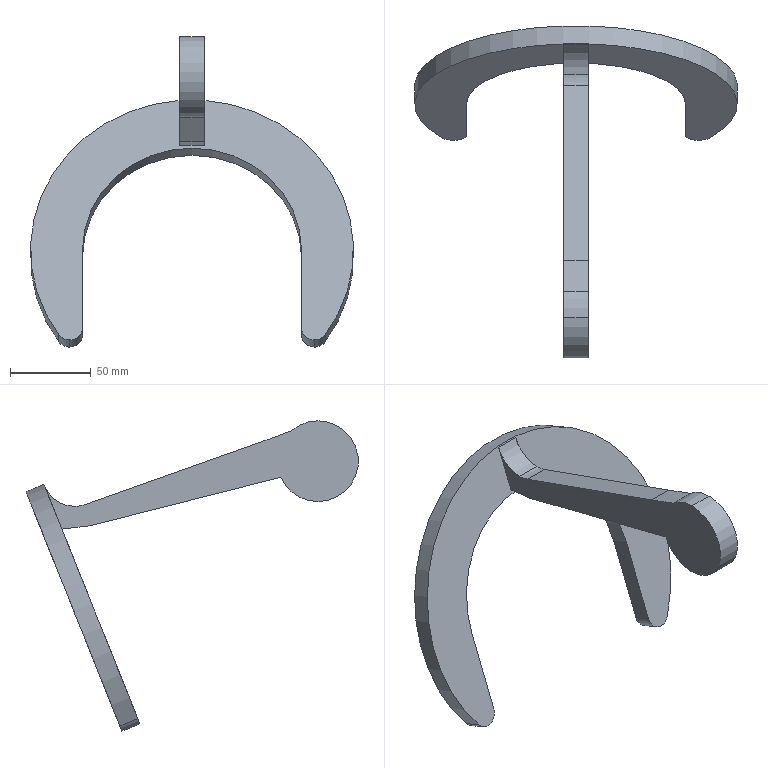Part | SolidWorks | features ICE 2, Extrusion 1, Fillet 1 | 1 solid | 21 faces | box 200 x 205.934 x 192.17 mm | volume 208238 mm3 | cylinder 11 | plane 10 | commonest cylinder face diameters 16 x4 50 x3 40 x2 135.704 x1 200 x1
STEP:
#1=CARTESIAN_POINT('',(-7.5,150.736,-27.917));
#2=VERTEX_POINT('',#1);
#3=CARTESIAN_POINT('',(-7.5,169.302,-15.355));
#4=VERTEX_POINT('',#3);
#5=CARTESIAN_POINT('',(-7.5,150.736,-7.917));
#6=DIRECTION('',(1.,0.,0.));
#7=DIRECTION('',(0.,0.,-1.));
#8=AXIS2_PLACEMENT_3D('',#5,#6,#7);
#9=CIRCLE('',#8,20.);
#10=EDGE_CURVE('',#2,#4,#9,.T.);
#11=ORIENTED_EDGE('',*,*,#10,.F.);
#12=CARTESIAN_POINT('',(7.5,150.736,-27.917));
#13=VERTEX_POINT('',#12);
#14=CARTESIAN_POINT('',(7.5,150.736,-27.917));
#15=DIRECTION('',(1.,0.,0.));
#16=VECTOR('',#15,1000.);
#17=LINE('',#14,#16);
#18=EDGE_CURVE('',#2,#13,#17,.T.);
#19=ORIENTED_EDGE('',*,*,#18,.T.);
#20=CARTESIAN_POINT('',(7.5,169.302,-15.355));
#21=VERTEX_POINT('',#20);
#22=CARTESIAN_POINT('',(7.5,150.736,-7.917));
#23=DIRECTION('',(-1.,0.,0.));
#24=DIRECTION('',(0.,0.,-1.));
#25=AXIS2_PLACEMENT_3D('',#22,#23,#24);
#26=CIRCLE('',#25,20.);
#27=EDGE_CURVE('',#21,#13,#26,.T.);
#28=ORIENTED_EDGE('',*,*,#27,.F.);
#29=CARTESIAN_POINT('',(7.5,169.302,-15.355));
#30=DIRECTION('',(1.,0.,0.));
#31=VECTOR('',#30,1000.);
#32=LINE('',#29,#31);
#33=EDGE_CURVE('',#4,#21,#32,.T.);
#34=ORIENTED_EDGE('',*,*,#33,.F.);
#35=EDGE_LOOP('',(#11,#19,#28,#34));
#36=FACE_OUTER_BOUND('',#35,.T.);
#37=CARTESIAN_POINT('',(7.5,150.736,-7.917));
#38=DIRECTION('',(1.,0.,0.));
#39=DIRECTION('',(0.,0.,-1.));
#40=AXIS2_PLACEMENT_3D('',#37,#38,#39);
#41=CYLINDRICAL_SURFACE('',#40,20.);
#42=ADVANCED_FACE('',(#36),#41,.F.);
#43=CARTESIAN_POINT('',(75.852,121.408,-167.17));
#44=VERTEX_POINT('',#43);
#45=CARTESIAN_POINT('',(67.852,124.383,-159.743));
#46=VERTEX_POINT('',#45);
#47=CARTESIAN_POINT('',(75.852,124.383,-159.743));
#48=DIRECTION('',(0.,0.9283,-0.3719));
#49=DIRECTION('',(0.,-0.3719,-0.9283));
#50=AXIS2_PLACEMENT_3D('',#47,#48,#49);
#51=CIRCLE('',#50,8.);
#52=EDGE_CURVE('',#44,#46,#51,.T.);
#53=ORIENTED_EDGE('',*,*,#52,.F.);
#54=CARTESIAN_POINT('',(75.852,110.269,-162.707));
#55=VERTEX_POINT('',#54);
#56=CARTESIAN_POINT('',(75.852,121.408,-167.17));
#57=DIRECTION('',(0.,-0.9283,0.3719));
#58=VECTOR('',#57,1000.);
#59=LINE('',#56,#58);
#60=EDGE_CURVE('',#44,#55,#59,.T.);
#61=ORIENTED_EDGE('',*,*,#60,.T.);
#62=CARTESIAN_POINT('',(67.852,113.244,-155.281));
#63=VERTEX_POINT('',#62);
#64=CARTESIAN_POINT('',(75.852,113.244,-155.281));
#65=DIRECTION('',(0.,0.9283,-0.3719));
#66=DIRECTION('',(0.,-0.3719,-0.9283));
#67=AXIS2_PLACEMENT_3D('',#64,#65,#66);
#68=CIRCLE('',#67,8.);
#69=EDGE_CURVE('',#55,#63,#68,.T.);
#70=ORIENTED_EDGE('',*,*,#69,.T.);
#71=CARTESIAN_POINT('',(67.852,124.383,-159.743));
#72=DIRECTION('',(0.,-0.9283,0.3719));
#73=VECTOR('',#72,1000.);
#74=LINE('',#71,#73);
#75=EDGE_CURVE('',#46,#63,#74,.T.);
#76=ORIENTED_EDGE('',*,*,#75,.F.);
#77=EDGE_LOOP('',(#53,#61,#70,#76));
#78=FACE_OUTER_BOUND('',#77,.T.);
#79=CARTESIAN_POINT('',(75.852,124.383,-159.743));
#80=DIRECTION('',(0.,-0.9283,0.3719));
#81=DIRECTION('',(0.,-0.3719,-0.9283));
#82=AXIS2_PLACEMENT_3D('',#79,#80,#81);
#83=CYLINDRICAL_SURFACE('',#82,8.);
#84=ADVANCED_FACE('',(#78),#83,.T.);
#85=CARTESIAN_POINT('',(-75.852,121.408,-167.17));
#86=VERTEX_POINT('',#85);
#87=CARTESIAN_POINT('',(-82.448,122.7,-163.946));
#88=VERTEX_POINT('',#87);
#89=CARTESIAN_POINT('',(-75.852,124.383,-159.743));
#90=DIRECTION('',(0.,0.9283,-0.3719));
#91=DIRECTION('',(0.,0.3719,0.9283));
#92=AXIS2_PLACEMENT_3D('',#89,#90,#91);
#93=CIRCLE('',#92,8.);
#94=EDGE_CURVE('',#86,#88,#93,.T.);
#95=ORIENTED_EDGE('',*,*,#94,.F.);
#96=CARTESIAN_POINT('',(-75.852,110.269,-162.707));
#97=VERTEX_POINT('',#96);
#98=CARTESIAN_POINT('',(-75.852,121.408,-167.17));
#99=DIRECTION('',(0.,-0.9283,0.3719));
#100=VECTOR('',#99,1000.);
#101=LINE('',#98,#100);
#102=EDGE_CURVE('',#86,#97,#101,.T.);
#103=ORIENTED_EDGE('',*,*,#102,.T.);
#104=CARTESIAN_POINT('',(-82.448,111.56,-159.483));
#105=VERTEX_POINT('',#104);
#106=CARTESIAN_POINT('',(-75.852,113.244,-155.281));
#107=DIRECTION('',(0.,0.9283,-0.3719));
#108=DIRECTION('',(0.,0.3719,0.9283));
#109=AXIS2_PLACEMENT_3D('',#106,#107,#108);
#110=CIRCLE('',#109,8.);
#111=EDGE_CURVE('',#97,#105,#110,.T.);
#112=ORIENTED_EDGE('',*,*,#111,.T.);
#113=CARTESIAN_POINT('',(-82.448,122.7,-163.946));
#114=DIRECTION('',(0.,-0.9283,0.3719));
#115=VECTOR('',#114,1000.);
#116=LINE('',#113,#115);
#117=EDGE_CURVE('',#88,#105,#116,.T.);
#118=ORIENTED_EDGE('',*,*,#117,.F.);
#119=EDGE_LOOP('',(#95,#103,#112,#118));
#120=FACE_OUTER_BOUND('',#119,.T.);
#121=CARTESIAN_POINT('',(-75.852,124.383,-159.743));
#122=DIRECTION('',(0.,-0.9283,0.3719));
#123=DIRECTION('',(0.,-0.3719,-0.9283));
#124=AXIS2_PLACEMENT_3D('',#121,#122,#123);
#125=CYLINDRICAL_SURFACE('',#124,8.);
#126=ADVANCED_FACE('',(#120),#125,.T.);
#127=CARTESIAN_POINT('',(7.5,0.,-25.));
#128=VERTEX_POINT('',#127);
#129=CARTESIAN_POINT('',(7.5,22.922,-9.978));
#130=VERTEX_POINT('',#129);
#131=CARTESIAN_POINT('',(7.5,0.,0.));
#132=DIRECTION('',(1.,0.,0.));
#133=DIRECTION('',(0.,0.,-1.));
#134=AXIS2_PLACEMENT_3D('',#131,#132,#133);
#135=CIRCLE('',#134,25.);
#136=EDGE_CURVE('',#128,#130,#135,.T.);
#137=ORIENTED_EDGE('',*,*,#136,.F.);
#138=CARTESIAN_POINT('',(-7.5,0.,-25.));
#139=VERTEX_POINT('',#138);
#140=CARTESIAN_POINT('',(7.5,0.,-25.));
#141=DIRECTION('',(-1.,0.,0.));
#142=VECTOR('',#141,1000.);
#143=LINE('',#140,#142);
#144=EDGE_CURVE('',#128,#139,#143,.T.);
#145=ORIENTED_EDGE('',*,*,#144,.T.);
#146=CARTESIAN_POINT('',(-7.5,22.922,-9.978));
#147=VERTEX_POINT('',#146);
#148=CARTESIAN_POINT('',(-7.5,0.,0.));
#149=DIRECTION('',(1.,0.,0.));
#150=DIRECTION('',(0.,0.,-1.));
#151=AXIS2_PLACEMENT_3D('',#148,#149,#150);
#152=CIRCLE('',#151,25.);
#153=EDGE_CURVE('',#139,#147,#152,.T.);
#154=ORIENTED_EDGE('',*,*,#153,.T.);
#155=CARTESIAN_POINT('',(7.5,22.922,-9.978));
#156=DIRECTION('',(-1.,0.,0.));
#157=VECTOR('',#156,1000.);
#158=LINE('',#155,#157);
#159=EDGE_CURVE('',#130,#147,#158,.T.);
#160=ORIENTED_EDGE('',*,*,#159,.F.);
#161=EDGE_LOOP('',(#137,#145,#154,#160));
#162=FACE_OUTER_BOUND('',#161,.T.);
#163=CARTESIAN_POINT('',(7.5,0.,0.));
#164=DIRECTION('',(-1.,0.,0.));
#165=DIRECTION('',(0.,0.,1.));
#166=AXIS2_PLACEMENT_3D('',#163,#164,#165);
#167=CYLINDRICAL_SURFACE('',#166,25.);
#168=ADVANCED_FACE('',(#162),#167,.T.);
#169=ORIENTED_EDGE('',*,*,#144,.F.);
#170=CARTESIAN_POINT('',(7.5,0.,25.));
#171=VERTEX_POINT('',#170);
#172=CARTESIAN_POINT('',(7.5,0.,0.));
#173=DIRECTION('',(1.,0.,0.));
#174=DIRECTION('',(0.,0.,-1.));
#175=AXIS2_PLACEMENT_3D('',#172,#173,#174);
#176=CIRCLE('',#175,25.);
#177=EDGE_CURVE('',#171,#128,#176,.T.);
#178=ORIENTED_EDGE('',*,*,#177,.F.);
#179=CARTESIAN_POINT('',(-7.5,0.,25.));
#180=VERTEX_POINT('',#179);
#181=CARTESIAN_POINT('',(7.5,0.,25.));
#182=DIRECTION('',(-1.,0.,0.));
#183=VECTOR('',#182,1000.);
#184=LINE('',#181,#183);
#185=EDGE_CURVE('',#171,#180,#184,.T.);
#186=ORIENTED_EDGE('',*,*,#185,.T.);
#187=CARTESIAN_POINT('',(-7.5,0.,0.));
#188=DIRECTION('',(1.,0.,0.));
#189=DIRECTION('',(0.,0.,-1.));
#190=AXIS2_PLACEMENT_3D('',#187,#188,#189);
#191=CIRCLE('',#190,25.);
#192=EDGE_CURVE('',#180,#139,#191,.T.);
#193=ORIENTED_EDGE('',*,*,#192,.T.);
#194=EDGE_LOOP('',(#169,#178,#186,#193));
#195=FACE_OUTER_BOUND('',#194,.T.);
#196=CARTESIAN_POINT('',(7.5,0.,0.));
#197=DIRECTION('',(-1.,0.,0.));
#198=DIRECTION('',(0.,0.,1.));
#199=AXIS2_PLACEMENT_3D('',#196,#197,#198);
#200=CYLINDRICAL_SURFACE('',#199,25.);
#201=ADVANCED_FACE('',(#195),#200,.T.);
#202=ORIENTED_EDGE('',*,*,#185,.F.);
#203=CARTESIAN_POINT('',(7.5,16.342,18.92));
#204=VERTEX_POINT('',#203);
#205=CARTESIAN_POINT('',(7.5,0.,0.));
#206=DIRECTION('',(1.,0.,0.));
#207=DIRECTION('',(0.,0.,-1.));
#208=AXIS2_PLACEMENT_3D('',#205,#206,#207);
#209=CIRCLE('',#208,25.);
#210=EDGE_CURVE('',#204,#171,#209,.T.);
#211=ORIENTED_EDGE('',*,*,#210,.F.);
#212=CARTESIAN_POINT('',(-7.5,16.342,18.92));
#213=VERTEX_POINT('',#212);
#214=CARTESIAN_POINT('',(7.5,16.342,18.92));
#215=DIRECTION('',(1.,0.,0.));
#216=VECTOR('',#215,1000.);
#217=LINE('',#214,#216);
#218=EDGE_CURVE('',#213,#204,#217,.T.);
#219=ORIENTED_EDGE('',*,*,#218,.F.);
#220=CARTESIAN_POINT('',(-7.5,0.,0.));
#221=DIRECTION('',(1.,0.,0.));
#222=DIRECTION('',(0.,0.,-1.));
#223=AXIS2_PLACEMENT_3D('',#220,#221,#222);
#224=CIRCLE('',#223,25.);
#225=EDGE_CURVE('',#213,#180,#224,.T.);
#226=ORIENTED_EDGE('',*,*,#225,.T.);
#227=EDGE_LOOP('',(#202,#211,#219,#226));
#228=FACE_OUTER_BOUND('',#227,.T.);
#229=CARTESIAN_POINT('',(7.5,0.,0.));
#230=DIRECTION('',(-1.,0.,0.));
#231=DIRECTION('',(0.,0.,1.));
#232=AXIS2_PLACEMENT_3D('',#229,#230,#231);
#233=CYLINDRICAL_SURFACE('',#232,25.);
#234=ADVANCED_FACE('',(#228),#233,.T.);
#235=ORIENTED_EDGE('',*,*,#210,.T.);
#236=ORIENTED_EDGE('',*,*,#177,.T.);
#237=ORIENTED_EDGE('',*,*,#136,.T.);
#238=CARTESIAN_POINT('',(7.5,141.125,-39.917));
#239=VERTEX_POINT('',#238);
#240=CARTESIAN_POINT('',(7.5,-2.,-3.666));
#241=DIRECTION('',(0.,0.9694,-0.2455));
#242=VECTOR('',#241,1000.);
#243=LINE('',#240,#242);
#244=EDGE_CURVE('',#130,#239,#243,.T.);
#245=ORIENTED_EDGE('',*,*,#244,.T.);
#246=CARTESIAN_POINT('',(7.5,158.581,-42.115));
#247=VERTEX_POINT('',#246);
#248=CARTESIAN_POINT('',(7.5,141.125,-39.917));
#249=DIRECTION('',(0.,0.9922,-0.1249));
#250=VECTOR('',#249,1000.);
#251=LINE('',#248,#250);
#252=EDGE_CURVE('',#239,#247,#251,.T.);
#253=ORIENTED_EDGE('',*,*,#252,.T.);
#254=CARTESIAN_POINT('',(7.5,158.581,-42.115));
#255=DIRECTION('',(0.,0.3719,0.9283));
#256=VECTOR('',#255,1000.);
#257=LINE('',#254,#256);
#258=EDGE_CURVE('',#247,#21,#257,.T.);
#259=ORIENTED_EDGE('',*,*,#258,.T.);
#260=ORIENTED_EDGE('',*,*,#27,.T.);
#261=CARTESIAN_POINT('',(7.5,144.041,-26.763));
#262=VERTEX_POINT('',#261);
#263=CARTESIAN_POINT('',(7.5,150.736,-7.917));
#264=DIRECTION('',(-1.,0.,0.));
#265=DIRECTION('',(0.,0.,-1.));
#266=AXIS2_PLACEMENT_3D('',#263,#264,#265);
#267=CIRCLE('',#266,20.);
#268=EDGE_CURVE('',#13,#262,#267,.T.);
#269=ORIENTED_EDGE('',*,*,#268,.T.);
#270=CARTESIAN_POINT('',(7.5,35.334,11.853));
#271=VERTEX_POINT('',#270);
#272=CARTESIAN_POINT('',(7.5,35.334,11.853));
#273=DIRECTION('',(0.,-0.9423,0.3347));
#274=VECTOR('',#273,1000.);
#275=LINE('',#272,#274);
#276=EDGE_CURVE('',#262,#271,#275,.T.);
#277=ORIENTED_EDGE('',*,*,#276,.T.);
#278=CARTESIAN_POINT('',(7.5,0.,25.));
#279=DIRECTION('',(0.,-0.9372,0.3487));
#280=VECTOR('',#279,1000.);
#281=LINE('',#278,#280);
#282=EDGE_CURVE('',#271,#204,#281,.T.);
#283=ORIENTED_EDGE('',*,*,#282,.T.);
#284=EDGE_LOOP('',(#235,#236,#237,#245,#253,#259,#260,#269,#277,#283));
#285=FACE_OUTER_BOUND('',#284,.T.);
#286=CARTESIAN_POINT('',(7.5,0.,0.));
#287=DIRECTION('',(1.,0.,0.));
#288=DIRECTION('',(0.,0.,-1.));
#289=AXIS2_PLACEMENT_3D('',#286,#287,#288);
#290=PLANE('',#289);
#291=ADVANCED_FACE('',(#285),#290,.T.);
#292=CARTESIAN_POINT('',(-7.5,141.125,-39.917));
#293=VERTEX_POINT('',#292);
#294=CARTESIAN_POINT('',(-7.5,-2.,-3.666));
#295=DIRECTION('',(0.,0.9694,-0.2455));
#296=VECTOR('',#295,1000.);
#297=LINE('',#294,#296);
#298=EDGE_CURVE('',#147,#293,#297,.T.);
#299=ORIENTED_EDGE('',*,*,#298,.F.);
#300=ORIENTED_EDGE('',*,*,#153,.F.);
#301=ORIENTED_EDGE('',*,*,#192,.F.);
#302=ORIENTED_EDGE('',*,*,#225,.F.);
#303=CARTESIAN_POINT('',(-7.5,35.334,11.853));
#304=VERTEX_POINT('',#303);
#305=CARTESIAN_POINT('',(-7.5,0.,25.));
#306=DIRECTION('',(0.,-0.9372,0.3487));
#307=VECTOR('',#306,1000.);
#308=LINE('',#305,#307);
#309=EDGE_CURVE('',#304,#213,#308,.T.);
#310=ORIENTED_EDGE('',*,*,#309,.F.);
#311=CARTESIAN_POINT('',(-7.5,144.041,-26.763));
#312=VERTEX_POINT('',#311);
#313=CARTESIAN_POINT('',(-7.5,35.334,11.853));
#314=DIRECTION('',(0.,-0.9423,0.3347));
#315=VECTOR('',#314,1000.);
#316=LINE('',#313,#315);
#317=EDGE_CURVE('',#312,#304,#316,.T.);
#318=ORIENTED_EDGE('',*,*,#317,.F.);
#319=CARTESIAN_POINT('',(-7.5,150.736,-7.917));
#320=DIRECTION('',(1.,0.,0.));
#321=DIRECTION('',(0.,0.,-1.));
#322=AXIS2_PLACEMENT_3D('',#319,#320,#321);
#323=CIRCLE('',#322,20.);
#324=EDGE_CURVE('',#312,#2,#323,.T.);
#325=ORIENTED_EDGE('',*,*,#324,.T.);
#326=ORIENTED_EDGE('',*,*,#10,.T.);
#327=CARTESIAN_POINT('',(-7.5,158.581,-42.115));
#328=VERTEX_POINT('',#327);
#329=CARTESIAN_POINT('',(-7.5,158.581,-42.115));
#330=DIRECTION('',(0.,0.3719,0.9283));
#331=VECTOR('',#330,1000.);
#332=LINE('',#329,#331);
#333=EDGE_CURVE('',#328,#4,#332,.T.);
#334=ORIENTED_EDGE('',*,*,#333,.F.);
#335=CARTESIAN_POINT('',(-7.5,141.125,-39.917));
#336=DIRECTION('',(0.,0.9922,-0.1249));
#337=VECTOR('',#336,1000.);
#338=LINE('',#335,#337);
#339=EDGE_CURVE('',#293,#328,#338,.T.);
#340=ORIENTED_EDGE('',*,*,#339,.F.);
#341=EDGE_LOOP('',(#299,#300,#301,#302,#310,#318,#325,#326,#334,#340));
#342=FACE_OUTER_BOUND('',#341,.T.);
#343=CARTESIAN_POINT('',(-7.5,0.,0.));
#344=DIRECTION('',(1.,0.,0.));
#345=DIRECTION('',(0.,0.,-1.));
#346=AXIS2_PLACEMENT_3D('',#343,#344,#345);
#347=PLANE('',#346);
#348=ADVANCED_FACE('',(#342),#347,.F.);
#349=ORIENTED_EDGE('',*,*,#244,.F.);
#350=ORIENTED_EDGE('',*,*,#159,.T.);
#351=ORIENTED_EDGE('',*,*,#298,.T.);
#352=CARTESIAN_POINT('',(7.5,141.125,-39.917));
#353=DIRECTION('',(-1.,0.,0.));
#354=VECTOR('',#353,1000.);
#355=LINE('',#352,#354);
#356=EDGE_CURVE('',#239,#293,#355,.T.);
#357=ORIENTED_EDGE('',*,*,#356,.F.);
#358=EDGE_LOOP('',(#349,#350,#351,#357));
#359=FACE_OUTER_BOUND('',#358,.T.);
#360=CARTESIAN_POINT('',(7.5,-2.,-3.666));
#361=DIRECTION('',(0.,0.2455,0.9694));
#362=DIRECTION('',(0.,-0.9694,0.2455));
#363=AXIS2_PLACEMENT_3D('',#360,#361,#362);
#364=PLANE('',#363);
#365=ADVANCED_FACE('',(#359),#364,.F.);
#366=ORIENTED_EDGE('',*,*,#309,.T.);
#367=ORIENTED_EDGE('',*,*,#218,.T.);
#368=ORIENTED_EDGE('',*,*,#282,.F.);
#369=CARTESIAN_POINT('',(7.5,35.334,11.853));
#370=DIRECTION('',(-1.,0.,0.));
#371=VECTOR('',#370,1000.);
#372=LINE('',#369,#371);
#373=EDGE_CURVE('',#271,#304,#372,.T.);
#374=ORIENTED_EDGE('',*,*,#373,.T.);
#375=EDGE_LOOP('',(#366,#367,#368,#374));
#376=FACE_OUTER_BOUND('',#375,.T.);
#377=CARTESIAN_POINT('',(7.5,0.,25.));
#378=DIRECTION('',(0.,-0.3487,-0.9372));
#379=DIRECTION('',(0.,0.9372,-0.3487));
#380=AXIS2_PLACEMENT_3D('',#377,#378,#379);
#381=PLANE('',#380);
#382=ADVANCED_FACE('',(#376),#381,.F.);
#383=ORIENTED_EDGE('',*,*,#339,.T.);
#384=CARTESIAN_POINT('',(7.5,158.581,-42.115));
#385=DIRECTION('',(-1.,0.,0.));
#386=VECTOR('',#385,1000.);
#387=LINE('',#384,#386);
#388=EDGE_CURVE('',#247,#328,#387,.T.);
#389=ORIENTED_EDGE('',*,*,#388,.F.);
#390=ORIENTED_EDGE('',*,*,#252,.F.);
#391=ORIENTED_EDGE('',*,*,#356,.T.);
#392=EDGE_LOOP('',(#383,#389,#390,#391));
#393=FACE_OUTER_BOUND('',#392,.T.);
#394=CARTESIAN_POINT('',(7.5,141.125,-39.917));
#395=DIRECTION('',(0.,0.1249,0.9922));
#396=DIRECTION('',(0.,-0.9922,0.1249));
#397=AXIS2_PLACEMENT_3D('',#394,#395,#396);
#398=PLANE('',#397);
#399=ADVANCED_FACE('',(#393),#398,.F.);
#400=ORIENTED_EDGE('',*,*,#276,.F.);
#401=CARTESIAN_POINT('',(-7.5,144.041,-26.763));
#402=DIRECTION('',(-1.,0.,0.));
#403=VECTOR('',#402,1000.);
#404=LINE('',#401,#403);
#405=EDGE_CURVE('',#262,#312,#404,.T.);
#406=ORIENTED_EDGE('',*,*,#405,.T.);
#407=ORIENTED_EDGE('',*,*,#317,.T.);
#408=ORIENTED_EDGE('',*,*,#373,.F.);
#409=EDGE_LOOP('',(#400,#406,#407,#408));
#410=FACE_OUTER_BOUND('',#409,.T.);
#411=CARTESIAN_POINT('',(7.5,35.334,11.853));
#412=DIRECTION('',(0.,-0.3347,-0.9423));
#413=DIRECTION('',(0.,0.9423,-0.3347));
#414=AXIS2_PLACEMENT_3D('',#411,#412,#413);
#415=PLANE('',#414);
#416=ADVANCED_FACE('',(#410),#415,.F.);
#417=CARTESIAN_POINT('',(-67.852,113.244,-155.281));
#418=VERTEX_POINT('',#417);
#419=CARTESIAN_POINT('',(-75.852,113.244,-155.281));
#420=DIRECTION('',(0.,0.9283,-0.3719));
#421=DIRECTION('',(0.,0.3719,0.9283));
#422=AXIS2_PLACEMENT_3D('',#419,#420,#421);
#423=CIRCLE('',#422,8.);
#424=EDGE_CURVE('',#418,#97,#423,.T.);
#425=ORIENTED_EDGE('',*,*,#424,.F.);
#426=CARTESIAN_POINT('',(-67.852,132.605,-106.953));
#427=VERTEX_POINT('',#426);
#428=CARTESIAN_POINT('',(-67.852,113.244,-155.281));
#429=DIRECTION('',(0.,-0.3719,-0.9283));
#430=VECTOR('',#429,1000.);
#431=LINE('',#428,#430);
#432=EDGE_CURVE('',#427,#418,#431,.T.);
#433=ORIENTED_EDGE('',*,*,#432,.F.);
#434=CARTESIAN_POINT('',(67.852,132.605,-106.953));
#435=VERTEX_POINT('',#434);
#436=CARTESIAN_POINT('',(0.,132.605,-106.953));
#437=DIRECTION('',(0.,-0.9283,0.3719));
#438=DIRECTION('',(0.,0.3719,0.9283));
#439=AXIS2_PLACEMENT_3D('',#436,#437,#438);
#440=CIRCLE('',#439,67.852);
#441=EDGE_CURVE('',#435,#427,#440,.T.);
#442=ORIENTED_EDGE('',*,*,#441,.F.);
#443=CARTESIAN_POINT('',(67.852,113.244,-155.281));
#444=DIRECTION('',(0.,0.3719,0.9283));
#445=VECTOR('',#444,1000.);
#446=LINE('',#443,#445);
#447=EDGE_CURVE('',#63,#435,#446,.T.);
#448=ORIENTED_EDGE('',*,*,#447,.F.);
#449=ORIENTED_EDGE('',*,*,#69,.F.);
#450=CARTESIAN_POINT('',(82.448,111.56,-159.483));
#451=VERTEX_POINT('',#450);
#452=CARTESIAN_POINT('',(75.852,113.244,-155.281));
#453=DIRECTION('',(0.,0.9283,-0.3719));
#454=DIRECTION('',(0.,-0.3719,-0.9283));
#455=AXIS2_PLACEMENT_3D('',#452,#453,#454);
#456=CIRCLE('',#455,8.);
#457=EDGE_CURVE('',#451,#55,#456,.T.);
#458=ORIENTED_EDGE('',*,*,#457,.F.);
#459=CARTESIAN_POINT('',(0.,132.605,-106.953));
#460=DIRECTION('',(0.,0.9283,-0.3719));
#461=DIRECTION('',(0.,0.3719,0.9283));
#462=AXIS2_PLACEMENT_3D('',#459,#460,#461);
#463=CIRCLE('',#462,100.);
#464=EDGE_CURVE('',#105,#451,#463,.T.);
#465=ORIENTED_EDGE('',*,*,#464,.F.);
#466=ORIENTED_EDGE('',*,*,#111,.F.);
#467=EDGE_LOOP('',(#425,#433,#442,#448,#449,#458,#465,#466));
#468=FACE_OUTER_BOUND('',#467,.T.);
#469=ORIENTED_EDGE('',*,*,#333,.T.);
#470=ORIENTED_EDGE('',*,*,#33,.T.);
#471=ORIENTED_EDGE('',*,*,#258,.F.);
#472=ORIENTED_EDGE('',*,*,#388,.T.);
#473=EDGE_LOOP('',(#469,#470,#471,#472));
#474=FACE_BOUND('',#473,.T.);
#475=CARTESIAN_POINT('',(-75.852,113.244,-155.281));
#476=DIRECTION('',(0.,0.9283,-0.3719));
#477=DIRECTION('',(0.,0.3719,0.9283));
#478=AXIS2_PLACEMENT_3D('',#475,#476,#477);
#479=PLANE('',#478);
#480=ADVANCED_FACE('',(#468,#474),#479,.F.);
#481=ORIENTED_EDGE('',*,*,#102,.F.);
#482=CARTESIAN_POINT('',(-67.852,124.383,-159.743));
#483=VERTEX_POINT('',#482);
#484=CARTESIAN_POINT('',(-75.852,124.383,-159.743));
#485=DIRECTION('',(0.,0.9283,-0.3719));
#486=DIRECTION('',(0.,0.3719,0.9283));
#487=AXIS2_PLACEMENT_3D('',#484,#485,#486);
#488=CIRCLE('',#487,8.);
#489=EDGE_CURVE('',#483,#86,#488,.T.);
#490=ORIENTED_EDGE('',*,*,#489,.F.);
#491=CARTESIAN_POINT('',(-67.852,124.383,-159.743));
#492=DIRECTION('',(0.,-0.9283,0.3719));
#493=VECTOR('',#492,1000.);
#494=LINE('',#491,#493);
#495=EDGE_CURVE('',#483,#418,#494,.T.);
#496=ORIENTED_EDGE('',*,*,#495,.T.);
#497=ORIENTED_EDGE('',*,*,#424,.T.);
#498=EDGE_LOOP('',(#481,#490,#496,#497));
#499=FACE_OUTER_BOUND('',#498,.T.);
#500=CARTESIAN_POINT('',(-75.852,124.383,-159.743));
#501=DIRECTION('',(0.,-0.9283,0.3719));
#502=DIRECTION('',(0.,-0.3719,-0.9283));
#503=AXIS2_PLACEMENT_3D('',#500,#501,#502);
#504=CYLINDRICAL_SURFACE('',#503,8.);
#505=ADVANCED_FACE('',(#499),#504,.T.);
#506=ORIENTED_EDGE('',*,*,#464,.T.);
#507=CARTESIAN_POINT('',(82.448,122.7,-163.946));
#508=VERTEX_POINT('',#507);
#509=CARTESIAN_POINT('',(82.448,122.7,-163.946));
#510=DIRECTION('',(0.,-0.9283,0.3719));
#511=VECTOR('',#510,1000.);
#512=LINE('',#509,#511);
#513=EDGE_CURVE('',#508,#451,#512,.T.);
#514=ORIENTED_EDGE('',*,*,#513,.F.);
#515=CARTESIAN_POINT('',(0.,143.745,-111.415));
#516=DIRECTION('',(0.,0.9283,-0.3719));
#517=DIRECTION('',(0.,0.3719,0.9283));
#518=AXIS2_PLACEMENT_3D('',#515,#516,#517);
#519=CIRCLE('',#518,100.);
#520=EDGE_CURVE('',#88,#508,#519,.T.);
#521=ORIENTED_EDGE('',*,*,#520,.F.);
#522=ORIENTED_EDGE('',*,*,#117,.T.);
#523=EDGE_LOOP('',(#506,#514,#521,#522));
#524=FACE_OUTER_BOUND('',#523,.T.);
#525=CARTESIAN_POINT('',(0.,143.745,-111.415));
#526=DIRECTION('',(0.,-0.9283,0.3719));
#527=DIRECTION('',(0.,-0.3719,-0.9283));
#528=AXIS2_PLACEMENT_3D('',#525,#526,#527);
#529=CYLINDRICAL_SURFACE('',#528,100.);
#530=ADVANCED_FACE('',(#524),#529,.T.);
#531=ORIENTED_EDGE('',*,*,#60,.F.);
#532=CARTESIAN_POINT('',(75.852,124.383,-159.743));
#533=DIRECTION('',(0.,0.9283,-0.3719));
#534=DIRECTION('',(0.,-0.3719,-0.9283));
#535=AXIS2_PLACEMENT_3D('',#532,#533,#534);
#536=CIRCLE('',#535,8.);
#537=EDGE_CURVE('',#508,#44,#536,.T.);
#538=ORIENTED_EDGE('',*,*,#537,.F.);
#539=ORIENTED_EDGE('',*,*,#513,.T.);
#540=ORIENTED_EDGE('',*,*,#457,.T.);
#541=EDGE_LOOP('',(#531,#538,#539,#540));
#542=FACE_OUTER_BOUND('',#541,.T.);
#543=CARTESIAN_POINT('',(75.852,124.383,-159.743));
#544=DIRECTION('',(0.,-0.9283,0.3719));
#545=DIRECTION('',(0.,-0.3719,-0.9283));
#546=AXIS2_PLACEMENT_3D('',#543,#544,#545);
#547=CYLINDRICAL_SURFACE('',#546,8.);
#548=ADVANCED_FACE('',(#542),#547,.T.);
#549=ORIENTED_EDGE('',*,*,#447,.T.);
#550=CARTESIAN_POINT('',(67.852,143.745,-111.415));
#551=VERTEX_POINT('',#550);
#552=CARTESIAN_POINT('',(67.852,143.745,-111.415));
#553=DIRECTION('',(0.,-0.9283,0.3719));
#554=VECTOR('',#553,1000.);
#555=LINE('',#552,#554);
#556=EDGE_CURVE('',#551,#435,#555,.T.);
#557=ORIENTED_EDGE('',*,*,#556,.F.);
#558=CARTESIAN_POINT('',(67.852,124.383,-159.743));
#559=DIRECTION('',(0.,0.3719,0.9283));
#560=VECTOR('',#559,1000.);
#561=LINE('',#558,#560);
#562=EDGE_CURVE('',#46,#551,#561,.T.);
#563=ORIENTED_EDGE('',*,*,#562,.F.);
#564=ORIENTED_EDGE('',*,*,#75,.T.);
#565=EDGE_LOOP('',(#549,#557,#563,#564));
#566=FACE_OUTER_BOUND('',#565,.T.);
#567=CARTESIAN_POINT('',(67.852,124.383,-159.743));
#568=DIRECTION('',(1.,0.,0.));
#569=DIRECTION('',(0.,0.,-1.));
#570=AXIS2_PLACEMENT_3D('',#567,#568,#569);
#571=PLANE('',#570);
#572=ADVANCED_FACE('',(#566),#571,.F.);
#573=ORIENTED_EDGE('',*,*,#441,.T.);
#574=CARTESIAN_POINT('',(-67.852,143.745,-111.415));
#575=VERTEX_POINT('',#574);
#576=CARTESIAN_POINT('',(-67.852,143.745,-111.415));
#577=DIRECTION('',(0.,-0.9283,0.3719));
#578=VECTOR('',#577,1000.);
#579=LINE('',#576,#578);
#580=EDGE_CURVE('',#575,#427,#579,.T.);
#581=ORIENTED_EDGE('',*,*,#580,.F.);
#582=CARTESIAN_POINT('',(0.,143.745,-111.415));
#583=DIRECTION('',(0.,-0.9283,0.3719));
#584=DIRECTION('',(0.,0.3719,0.9283));
#585=AXIS2_PLACEMENT_3D('',#582,#583,#584);
#586=CIRCLE('',#585,67.852);
#587=EDGE_CURVE('',#551,#575,#586,.T.);
#588=ORIENTED_EDGE('',*,*,#587,.F.);
#589=ORIENTED_EDGE('',*,*,#556,.T.);
#590=EDGE_LOOP('',(#573,#581,#588,#589));
#591=FACE_OUTER_BOUND('',#590,.T.);
#592=CARTESIAN_POINT('',(0.,143.745,-111.415));
#593=DIRECTION('',(0.,-0.9283,0.3719));
#594=DIRECTION('',(0.,-0.3719,-0.9283));
#595=AXIS2_PLACEMENT_3D('',#592,#593,#594);
#596=CYLINDRICAL_SURFACE('',#595,67.852);
#597=ADVANCED_FACE('',(#591),#596,.F.);
#598=ORIENTED_EDGE('',*,*,#432,.T.);
#599=ORIENTED_EDGE('',*,*,#495,.F.);
#600=CARTESIAN_POINT('',(-67.852,124.383,-159.743));
#601=DIRECTION('',(0.,-0.3719,-0.9283));
#602=VECTOR('',#601,1000.);
#603=LINE('',#600,#602);
#604=EDGE_CURVE('',#575,#483,#603,.T.);
#605=ORIENTED_EDGE('',*,*,#604,.F.);
#606=ORIENTED_EDGE('',*,*,#580,.T.);
#607=EDGE_LOOP('',(#598,#599,#605,#606));
#608=FACE_OUTER_BOUND('',#607,.T.);
#609=CARTESIAN_POINT('',(-67.852,124.383,-159.743));
#610=DIRECTION('',(-1.,0.,0.));
#611=DIRECTION('',(0.,0.,1.));
#612=AXIS2_PLACEMENT_3D('',#609,#610,#611);
#613=PLANE('',#612);
#614=ADVANCED_FACE('',(#608),#613,.F.);
#615=ORIENTED_EDGE('',*,*,#489,.T.);
#616=ORIENTED_EDGE('',*,*,#94,.T.);
#617=ORIENTED_EDGE('',*,*,#520,.T.);
#618=ORIENTED_EDGE('',*,*,#537,.T.);
#619=ORIENTED_EDGE('',*,*,#52,.T.);
#620=ORIENTED_EDGE('',*,*,#562,.T.);
#621=ORIENTED_EDGE('',*,*,#587,.T.);
#622=ORIENTED_EDGE('',*,*,#604,.T.);
#623=EDGE_LOOP('',(#615,#616,#617,#618,#619,#620,#621,#622));
#624=FACE_OUTER_BOUND('',#623,.T.);
#625=CARTESIAN_POINT('',(-75.852,124.383,-159.743));
#626=DIRECTION('',(0.,0.9283,-0.3719));
#627=DIRECTION('',(0.,0.3719,0.9283));
#628=AXIS2_PLACEMENT_3D('',#625,#626,#627);
#629=PLANE('',#628);
#630=ADVANCED_FACE('',(#624),#629,.T.);
#631=ORIENTED_EDGE('',*,*,#18,.F.);
#632=ORIENTED_EDGE('',*,*,#324,.F.);
#633=ORIENTED_EDGE('',*,*,#405,.F.);
#634=ORIENTED_EDGE('',*,*,#268,.F.);
#635=EDGE_LOOP('',(#631,#632,#633,#634));
#636=FACE_OUTER_BOUND('',#635,.T.);
#637=CARTESIAN_POINT('',(7.5,150.736,-7.917));
#638=DIRECTION('',(1.,0.,0.));
#639=DIRECTION('',(0.,0.,-1.));
#640=AXIS2_PLACEMENT_3D('',#637,#638,#639);
#641=CYLINDRICAL_SURFACE('',#640,20.);
#642=ADVANCED_FACE('',(#636),#641,.F.);
#643=CLOSED_SHELL('',(#42,#84,#126,#168,#201,#234,#291,#348,#365,#382,#399,#416,#480,#505,#530,#548,#572,#597,#614,#630,#642));
#644=MANIFOLD_SOLID_BREP('',#643);
#645=CARTESIAN_POINT('',(0.,0.,0.));
#646=DIRECTION('',(0.,0.,1.));
#647=DIRECTION('',(1.,0.,0.));
#648=AXIS2_PLACEMENT_3D('',#645,#646,#647);
#649=(LENGTH_UNIT()NAMED_UNIT(*)SI_UNIT(.MILLI.,.METRE.));
#650=UNCERTAINTY_MEASURE_WITH_UNIT(LENGTH_MEASURE(0.00001),#649,'','');
#651=(NAMED_UNIT(*)PLANE_ANGLE_UNIT()SI_UNIT($,.RADIAN.));
#652=(NAMED_UNIT(*)SI_UNIT($,.STERADIAN.)SOLID_ANGLE_UNIT());
#653=(GEOMETRIC_REPRESENTATION_CONTEXT(3)GLOBAL_UNCERTAINTY_ASSIGNED_CONTEXT((#650))GLOBAL_UNIT_ASSIGNED_CONTEXT((#649,#651,#652))REPRESENTATION_CONTEXT('',''));
#654=ADVANCED_BREP_SHAPE_REPRESENTATION('',(#644,#648),#653);